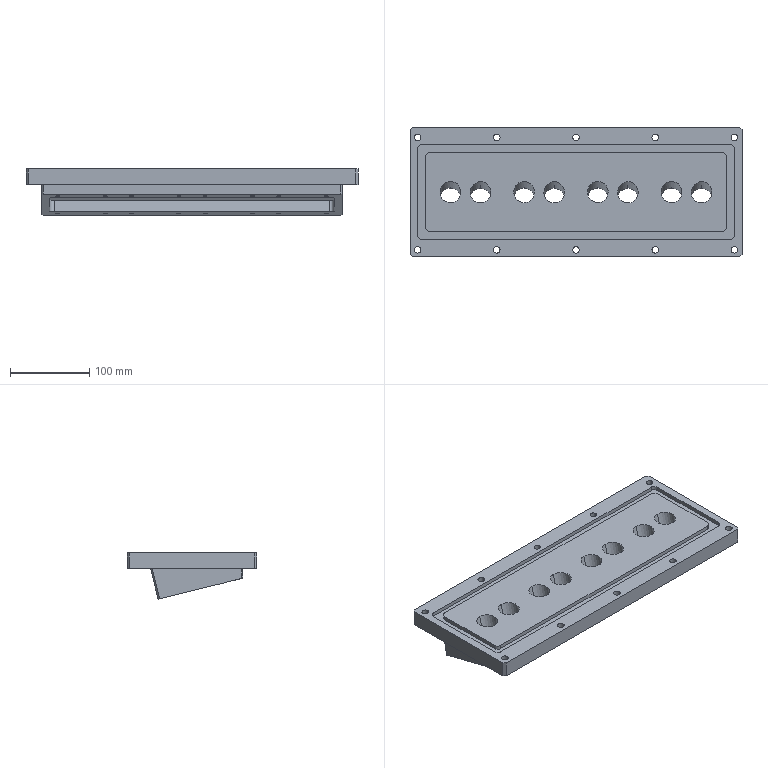Part | SolidWorks | features HoleWzd 3, ICE 3, Chamfer 2, Fillet 2, Extrusion 1 | 1 solid | 176 faces | box 419 x 164 x 58.51 mm | volume 1832163 mm3 | cylinder 100 | plane 44 | cone 32 | commonest cylinder face diameters 5 x32 8.4 x20 15 x20 26 x16 12 x12